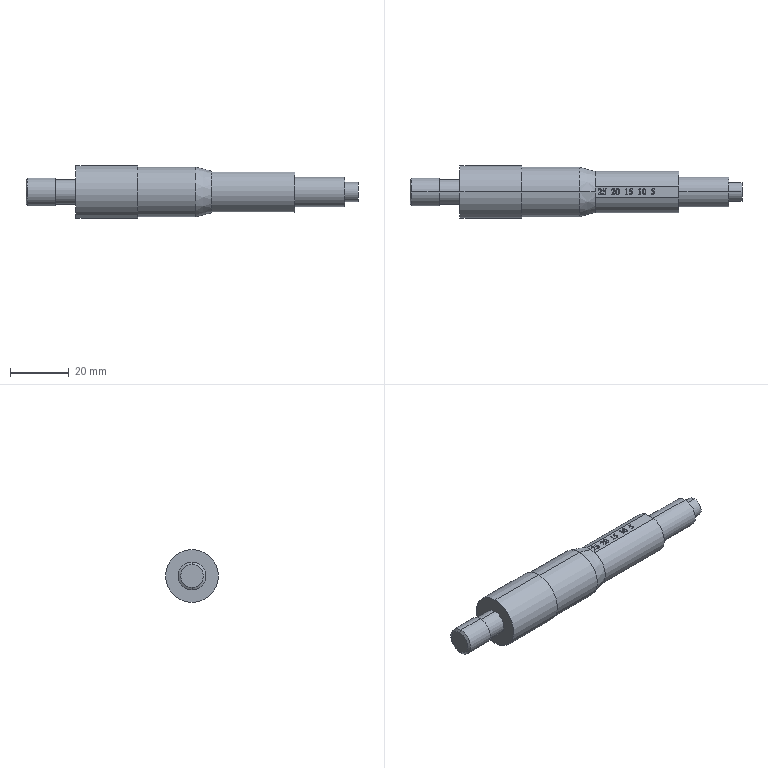Part | STEP file | Label: micrometer range 25mm diameter 12 new | 1 solid | 45 faces | box 113 x 18 x 18 mm | volume 13941 mm3 | plane 22 | cylinder 19 | cone 4 | commonest cylinder face diameters 6.5 x4 8.5 x2 9.5 x2 10 x2 12 x2 14.2 x2